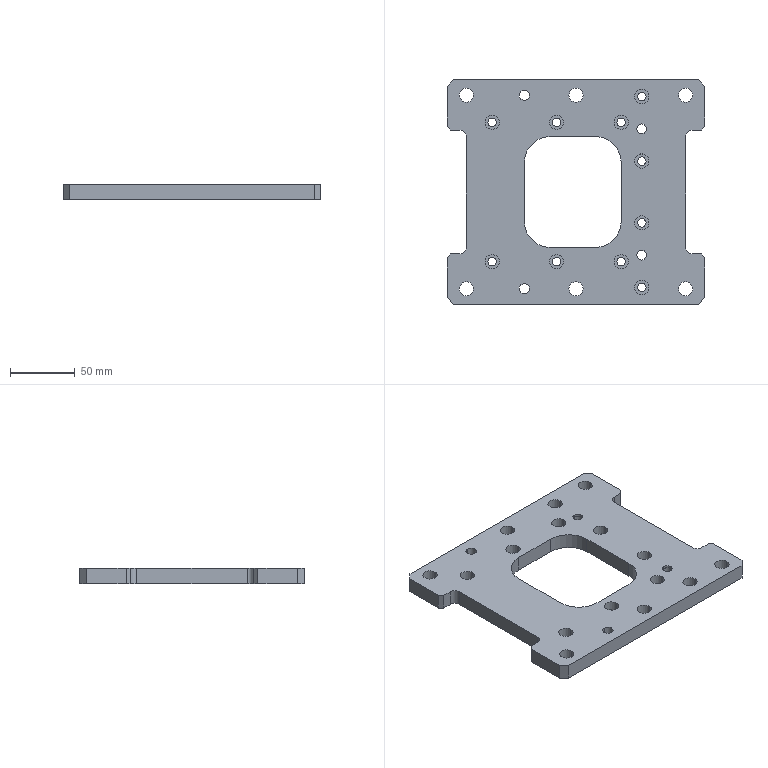Part | STEP file | J454-EBZ05-02-00-Part-1 | 1 solid | 110 faces | box 200 x 174 x 12 mm | volume 291304 mm3 | cylinder 72 | plane 38 | commonest cylinder face diameters 11 x32 6.6 x20 8 x8 7.5 x4 10 x4 40 x4